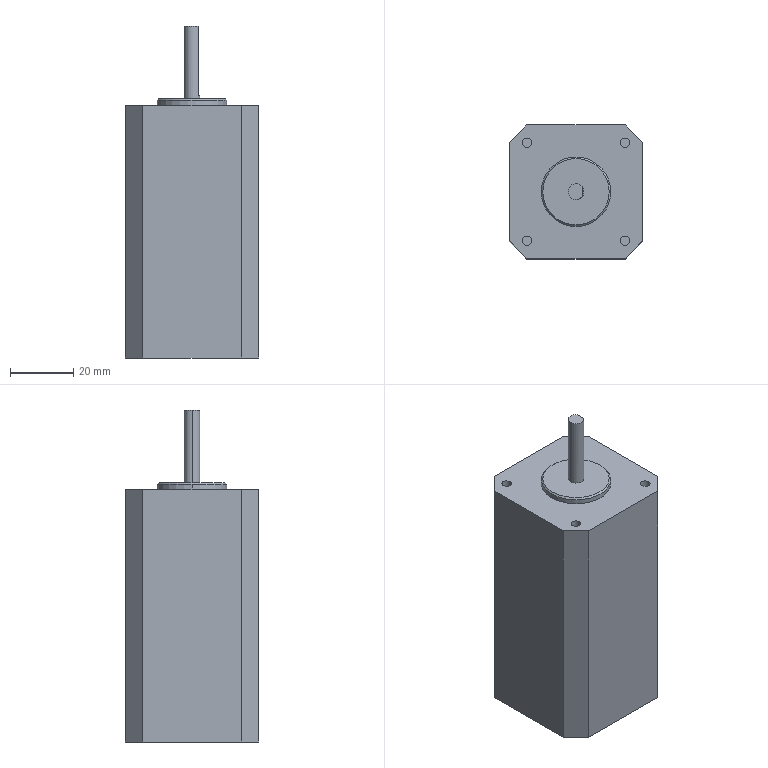Part | SolidWorks | features BaseBody 1 | 1 solid | 248 faces | box 42.3 x 42.3 x 105 mm | volume 139111 mm3 | plane 234 | cylinder 12 | cone 2 | commonest cylinder face diameters 3 x8 5 x2 22 x2